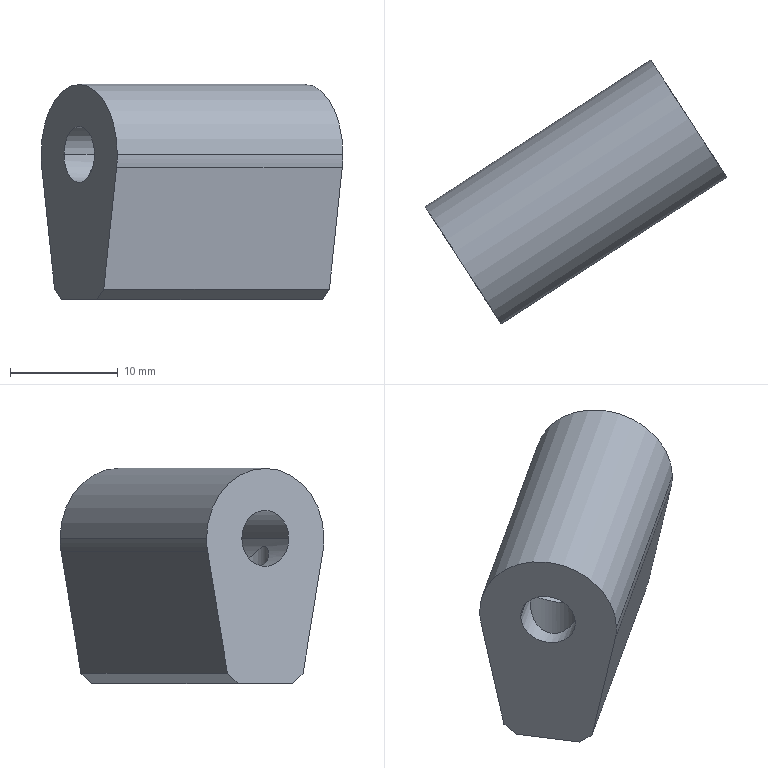Part | STEP file | GMBH_3A | 1 solid | 19 faces | box 28.047 x 24.519 x 20 mm | volume 4066 mm3 | cylinder 11 | plane 8 | commonest cylinder face diameters 5 x4 13 x3 5.2 x2 8.5 x2